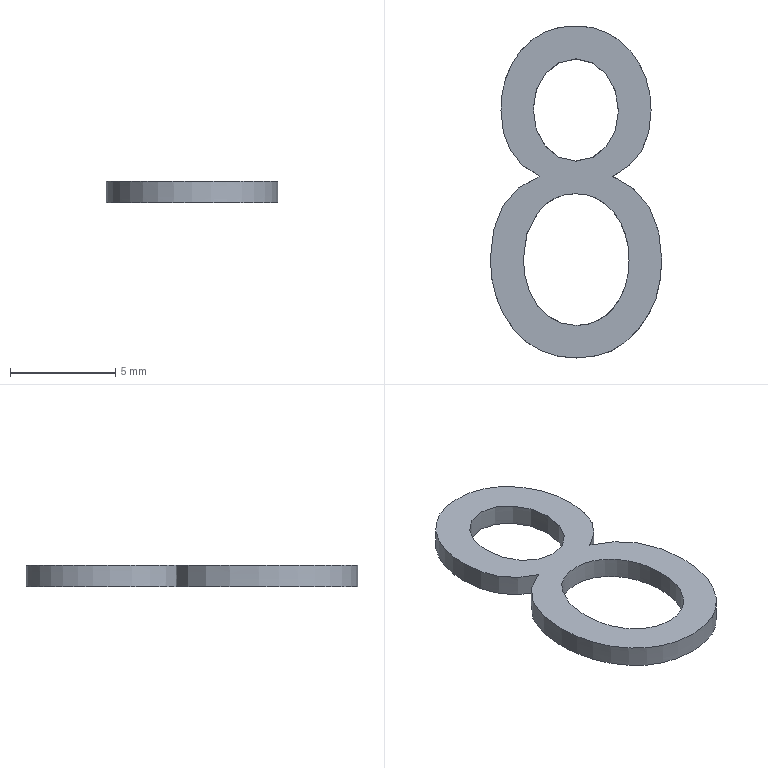Part | STEP file | lll_id1418_x_t | 1 solid | 5 faces | box 8.132 x 15.752 x 1 mm | volume 58.959 mm3 | other 3 | plane 2